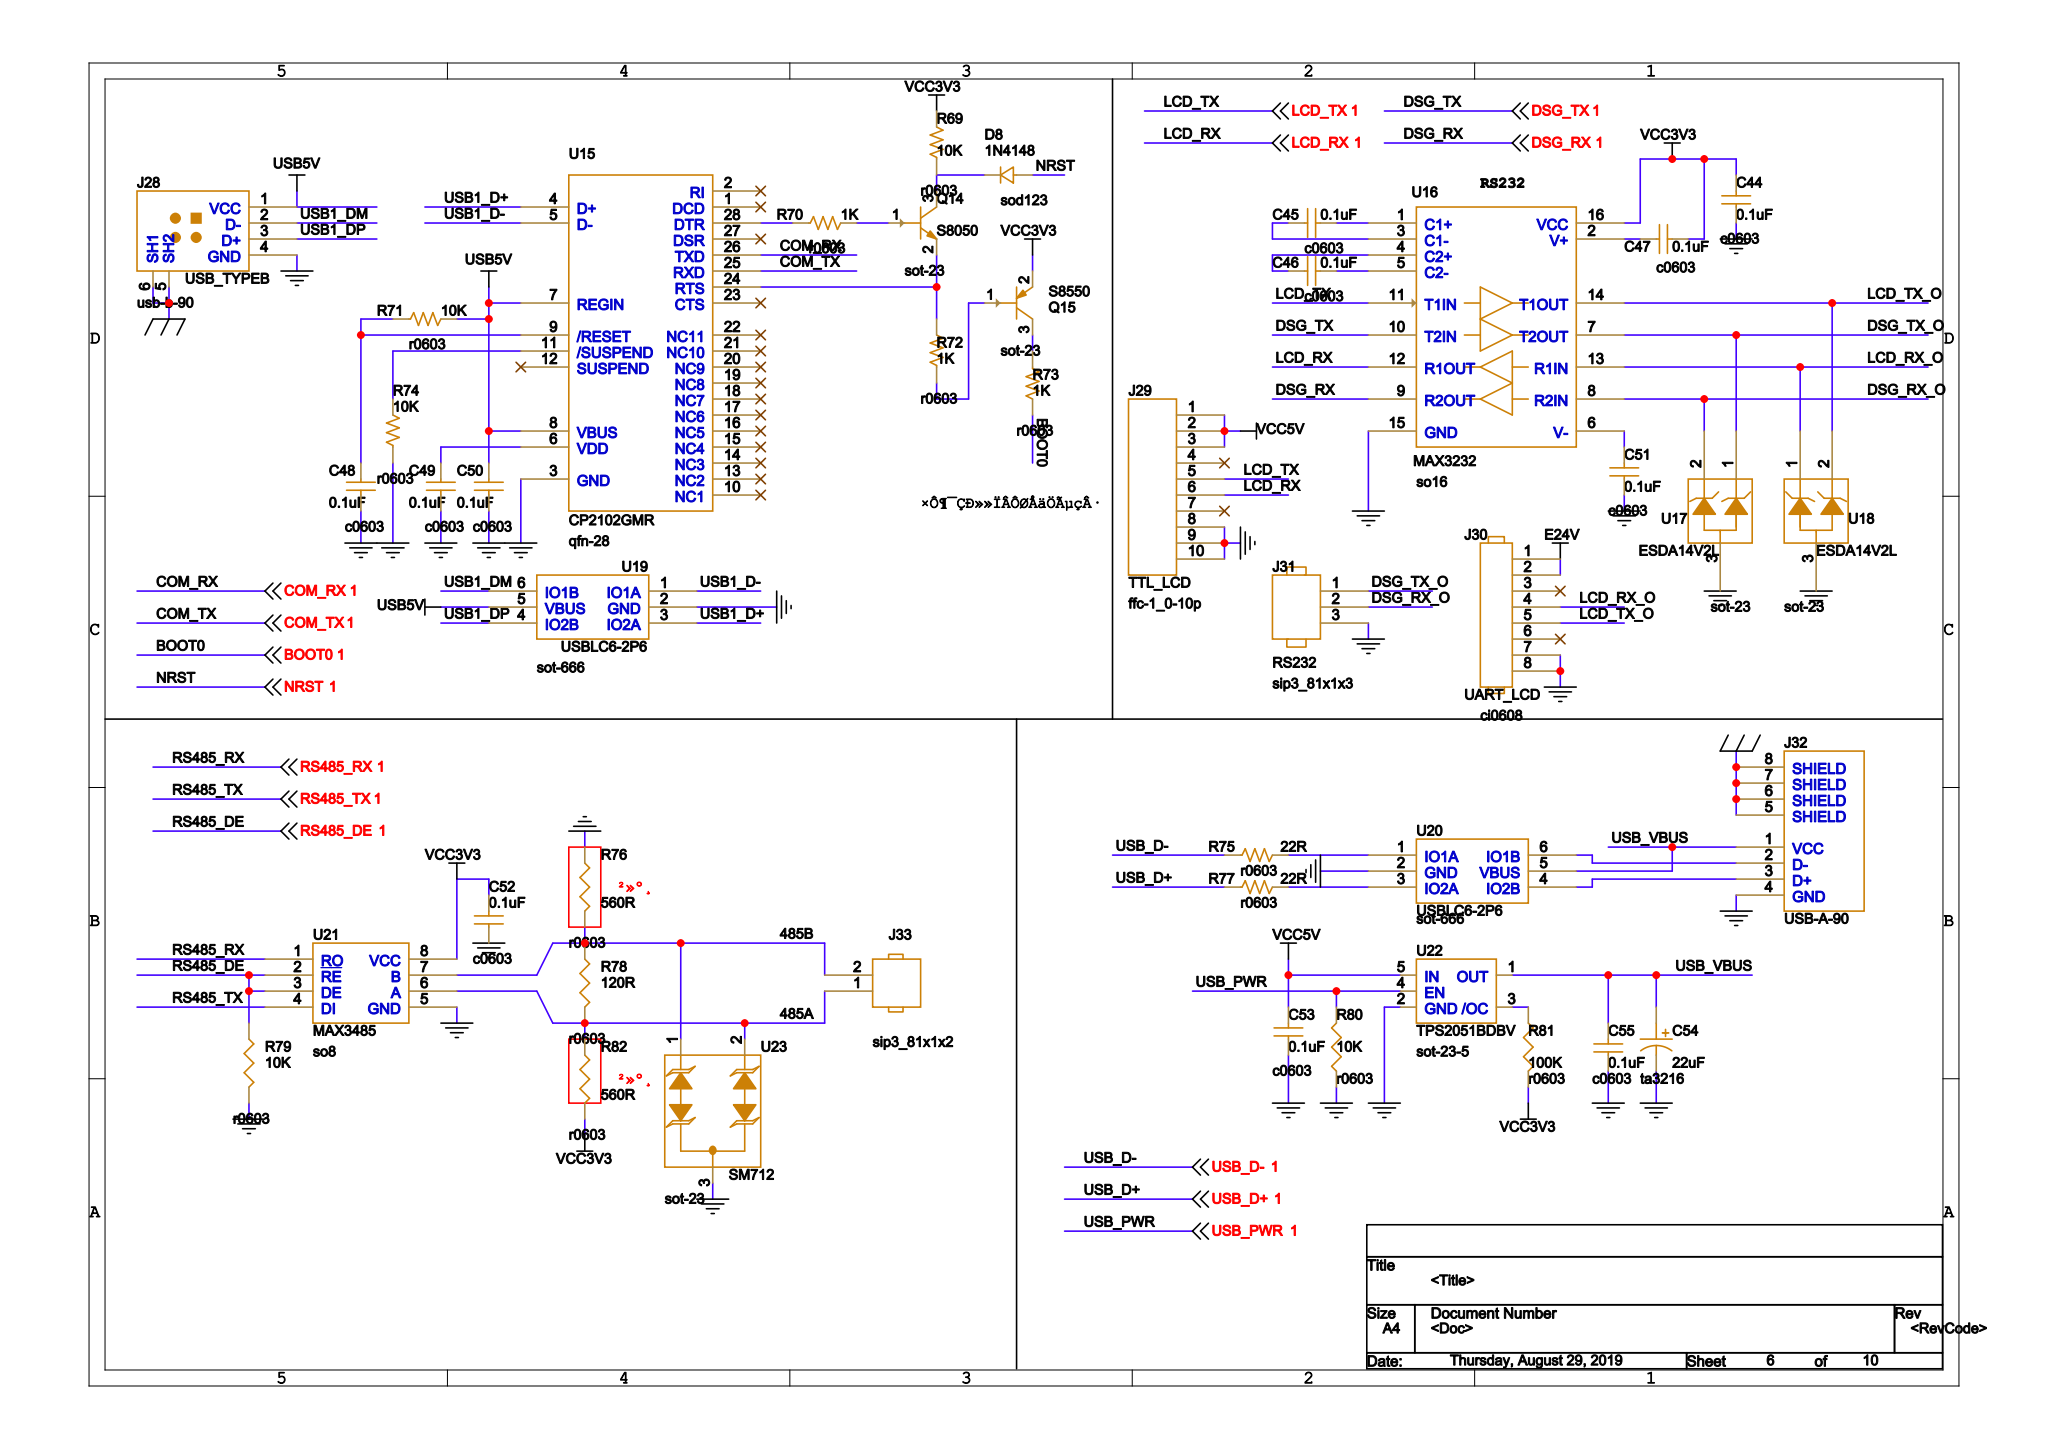Circuit board | Cadence Allegro | 380 parts | 375 nets | one sheet of the schematic
Parts on this sheet (reference | value | footprint):
C44 | 0.1uF | C0603
C45 | 0.1uF | C0603
C46 | 0.1uF | C0603
C47 | 0.1uF | C0603
C48 | 0.1uF | C0603
C49 | 0.1uF | C0603
C50 | 0.1uF | C0603
C51 | 0.1uF | C0603
C52 | 0.1uF | C0603
C53 | 0.1uF | C0603
C54 | 22uF | TA3216
C55 | 0.1uF | C0603
D8 | 1N4148 | SOD123
J28 | USB_TYPEB | USB-B-90
J29 | TTL_LCD | FFC-1_0-10P
J30 | UART_LCD | CI0608
J31 | RS232 | SIP3_81X1X3
J32 | USB-A-90 | USB-A-90
J33 | HEADER 2 | SIP3_81X1X2
Q14 | S8050 | SOT-23
Q15 | S8550 | SOT-23
R69 | 10K | R0603
R70 | 1K | R0603
R71 | 10K | R0603
R72 | 1K | R0603
R73 | 1K | R0603
R74 | 10K | R0603
R75 | 22R | R0603
R76 | 560R | R0603
R77 | 22R | R0603
R78 | 120R | R0603
R79 | 10K | R0603
R80 | 10K | R0603
R81 | 100K | R0603
R82 | 560R | R0603
U15 | CP2102GMR | QFN-28
U16 | MAX3232 | SO16
U17 | ESDA14V2L | SOT-23
U18 | ESDA14V2L | SOT-23
U19 | USBLC6-2P6 | SOT-666
U20 | USBLC6-2P6 | SOT-666
U21 | MAX3485 | SO8
U22 | TPS2051BDBV | SOT-23-5
U23 | SM712 | SOT-23
Nets of these parts (net: part-pin ...):
N1545718: J32-3 U20-4
N1545706: J32-2 U20-6
GND: C44-1 C48-2 C49-2 C50-2 C51-1 C52-1 C53-1 C54-2 C55-1 J28-4 J29-8 J29-9 J29-10 J30-7 J30-8 J31-3 J32-4 R74-1 R76-1 R79-2 R80-1 U15-3 U16-15 U17-3 U18-3 U19-2 U20-2 U21-5 U22-2 U23-3
GND_EARTH: J28-5 J28-6 J32-5 J32-6 J32-7 J32-8
USB_VBUS: C54-1 C55-2 J32-1 U20-5 U22-1
VCC3V3: C44-2 C47-2 C52-2 Q15-2 R69-2 R81-2 R82-2 U16-16 U21-8
N454135: C48-1 R71-1 U15-9
N454155: R74-2 U15-11
USB1_D+: U15-4 U19-3
USB1_D-: U15-5 U19-1
N1664625: R70-1 U15-28
USB5V: C50-1 J28-1 R71-2 U15-7 U15-8 U19-5
N1664839: Q14-2 R72-2 U15-24
COM_TX: U15-25
COM_RX: U15-26
N454249: C49-1 U15-6
VCC5V: C53-2 J29-1 J29-2 J29-3 U22-5
USB1_DP: J28-3 U19-4
USB1_DM: J28-2 U19-6
USB_D-: R75-1
N1545649: R75-2 U20-1
USB_D+: R77-1
N1545653: R77-2 U20-3
485B: J33-2 R76-2 R78-1 U21-7 U23-1
485A: J33-1 R78-2 R82-1 U21-6 U23-2
USB_PWR: R80-2 U22-4
E24V: J30-1 J30-2
N1541881: C45-2 U16-1
N1541953: C45-1 U16-3
N1541993: C46-1 U16-4
N1541965: C46-2 U16-5
LCD_RX_O: J30-4 U16-13 U18-1
LCD_RX: J29-6 U16-12
DSG_RX_O: J31-2 U16-8 U17-2
DSG_RX: U16-9
LCD_TX: J29-5 U16-11
LCD_TX_O: J30-5 U16-14 U18-2
DSG_TX: U16-10
DSG_TX_O: J31-1 U16-7 U17-1
N1542013: C47-1 U16-2
N1542109: C51-2 U16-6
RS485_DE: R79-1 U21-2 U21-3
RS485_TX: U21-4
RS485_RX: U21-1
N1544093: R81-1 U22-3
NRST: D8-1
N1664846: D8-2 Q14-3 R69-1
N1664696: Q14-1 R70-2
N1665321: Q15-1 R72-1
N1665353: Q15-3 R73-1
BOOT0: R73-2